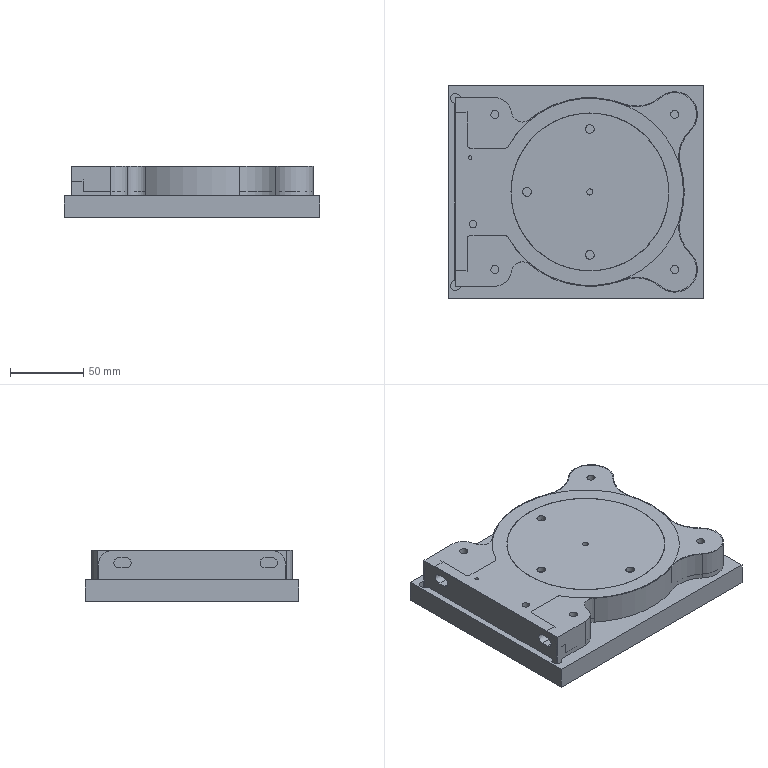NC program | NX | posted with a generic post | part box 175 x 146 x 35 mm
Lines 7000 to 8019 of 35144:
(深度开粗_COPY_COPY_1 , TOOL : D3)
N13836 T06 M6
N13838 G54
N13840 G17 G0 G90 X-69.928 Y23. S9000 M3
N13842 G43 Z20. H6
N13844 Z0.102
N13846 G94 G1 Z-0.398 F2500.
N13848 G3 X-71.428 Y24.5 R1.5
N13850 G1 X-72.5
N13852 G3 X-73. Y24. R0.5
N13854 G1 Y22.928
N13856 G3 X-71.5 Y21.428 R1.5
N13858 G1 Z0.102
N13860 G0 X-69.928 Y23. Z-0.296
N13862 G1 Z-0.796
N13864 G3 X-71.428 Y24.5 R1.5
N13866 G1 X-72.5
N13868 G3 X-73. Y24. R0.5
N13870 G1 Y22.928
N13872 G3 X-71.5 Y21.428 R1.5
N13874 G1 Z-0.296
N13876 G0 X-69.928 Y23. Z-0.694
N13878 G1 Z-1.194
N13880 G3 X-71.428 Y24.5 R1.5
N13882 G1 X-72.5
N13884 G3 X-73. Y24. R0.5
N13886 G1 Y22.928
N13888 G3 X-71.5 Y21.428 R1.5
N13890 G1 Z-0.694
N13892 G0 X-69.928 Y23. Z-1.092
N13894 G1 Z-1.592
N13896 G3 X-71.428 Y24.5 R1.5
N13898 G1 X-72.5
N13900 G3 X-73. Y24. R0.5
N13902 G1 Y22.928
N13904 G3 X-71.5 Y21.428 R1.5
N13906 G1 Z-1.092
N13908 G0 X-69.928 Y23. Z-1.49
N13910 G1 Z-1.99
N13912 G3 X-71.428 Y24.5 R1.5
N13914 G1 X-72.5
N13916 G3 X-73. Y24. R0.5
N13918 G1 Y22.928
N13920 G3 X-71.5 Y21.428 R1.5
N13922 G1 Z-1.49
N13924 G0 X-69.928 Y23. Z-1.888
N13926 G1 Z-2.388
N13928 G3 X-71.428 Y24.5 R1.5
N13930 G1 X-72.5
N13932 G3 X-73. Y24. R0.5
N13934 G1 Y22.928
N13936 G3 X-71.5 Y21.428 R1.5
N13938 G1 Z-1.888
N13940 G0 X-69.928 Y23. Z-2.286
N13942 G1 Z-2.786
N13944 G3 X-71.428 Y24.5 R1.5
N13946 G1 X-72.5
N13948 G3 X-73. Y24. R0.5
N13950 G1 Y22.928
N13952 G3 X-71.5 Y21.428 R1.5
N13954 G1 Z-2.286
N13956 G0 X-69.928 Y23. Z-2.684
N13958 G1 Z-3.184
N13960 G3 X-71.428 Y24.5 R1.5
N13962 G1 X-72.5
N13964 G3 X-73. Y24. R0.5
N13966 G1 Y22.928
N13968 G3 X-71.5 Y21.428 R1.5
N13970 G1 Z-2.684
N13972 G0 X-69.928 Y23. Z-3.082
N13974 G1 Z-3.582
N13976 G3 X-71.428 Y24.5 R1.5
N13978 G1 X-72.5
N13980 G3 X-73. Y24. R0.5
N13982 G1 Y22.928
N13984 G3 X-71.5 Y21.428 R1.5
N13986 G1 Z-3.082
N13988 G0 X-69.928 Y23. Z-3.48
N13990 G1 Z-3.98
N13992 G3 X-71.428 Y24.5 R1.5
N13994 G1 X-72.5
N13996 G3 X-73. Y24. R0.5
N13998 G1 Y22.928
N14000 G3 X-71.5 Y21.428 R1.5
N14002 G1 Z-3.48
N14004 G0 X-69.928 Y23. Z-3.878
N14006 G1 Z-4.378
N14008 G3 X-71.428 Y24.5 R1.5
N14010 G1 X-72.5
N14012 G3 X-73. Y24. R0.5
N14014 G1 Y22.928
N14016 G3 X-71.5 Y21.428 R1.5
N14018 G1 Z-3.878
N14020 G0 X-69.928 Y23. Z-4.276
N14022 G1 Z-4.776
N14024 G3 X-71.428 Y24.5 R1.5
N14026 G1 X-72.5
N14028 G3 X-73. Y24. R0.5
N14030 G1 Y22.928
N14032 G3 X-71.5 Y21.428 R1.5
N14034 G1 Z-4.276
N14036 G0 X-69.928 Y23. Z-4.675
N14038 G1 Z-5.175
N14040 G3 X-71.428 Y24.5 R1.5
N14042 G1 X-72.5
N14044 G3 X-73. Y24. R0.5
N14046 G1 Y22.928
N14048 G3 X-71.5 Y21.428 R1.5
N14050 G1 Z-4.675
N14052 G0 X-69.928 Y23. Z-5.073
N14054 G1 Z-5.573
N14056 G3 X-71.428 Y24.5 R1.5
N14058 G1 X-72.5
N14060 G3 X-73. Y24. R0.5
N14062 G1 Y22.928
N14064 G3 X-71.5 Y21.428 R1.5
N14066 G1 Z-5.073
N14068 G0 X-69.928 Y23. Z-5.471
N14070 G1 Z-5.971
N14072 G3 X-71.428 Y24.5 R1.5
N14074 G1 X-72.5
N14076 G3 X-73. Y24. R0.5
N14078 G1 Y22.928
N14080 G3 X-71.5 Y21.428 R1.5
N14082 G1 Z-5.471
N14084 G0 X-69.928 Y23. Z-5.869
N14086 G1 Z-6.369
N14088 G3 X-71.428 Y24.5 R1.5
N14090 G1 X-72.5
N14092 G3 X-73. Y24. R0.5
N14094 G1 Y22.928
N14096 G3 X-71.5 Y21.428 R1.5
N14098 G1 Z-5.869
N14100 G0 X-69.928 Y23. Z-6.267
N14102 G1 Z-6.767
N14104 G3 X-71.428 Y24.5 R1.5
N14106 G1 X-72.5
N14108 G3 X-73. Y24. R0.5
N14110 G1 Y22.928
N14112 G3 X-71.5 Y21.428 R1.5
N14114 G1 Z-6.267
N14116 G0 X-69.928 Y23. Z-6.665
N14118 G1 Z-7.165
N14120 G3 X-71.428 Y24.5 R1.5
N14122 G1 X-72.5
N14124 G3 X-73. Y24. R0.5
N14126 G1 Y22.928
N14128 G3 X-71.5 Y21.428 R1.5
N14130 G1 Z-6.665
N14132 G0 X-69.928 Y23. Z-7.063
N14134 G1 Z-7.563
N14136 G3 X-71.428 Y24.5 R1.5
N14138 G1 X-72.5
N14140 G3 X-73. Y24. R0.5
N14142 G1 Y22.928
N14144 G3 X-71.5 Y21.428 R1.5
N14146 G1 Z-7.063
N14148 G0 X-69.928 Y23. Z-7.461
N14150 G1 Z-7.961
N14152 G3 X-71.428 Y24.5 R1.5
N14154 G1 X-72.5
N14156 G3 X-73. Y24. R0.5
N14158 G1 Y22.928
N14160 G3 X-71.5 Y21.428 R1.5
N14162 G1 Z-7.461
N14164 G0 X-69.928 Y23. Z-7.859
N14166 G1 Z-8.359
N14168 G3 X-71.428 Y24.5 R1.5
N14170 G1 X-72.5
N14172 G3 X-73. Y24. R0.5
N14174 G1 Y22.928
N14176 G3 X-71.5 Y21.428 R1.5
N14178 G1 Z-7.859
N14180 G0 X-69.928 Y23. Z-8.257
N14182 G1 Z-8.757
N14184 G3 X-71.428 Y24.5 R1.5
N14186 G1 X-72.5
N14188 G3 X-73. Y24. R0.5
N14190 G1 Y22.928
N14192 G3 X-71.5 Y21.428 R1.5
N14194 G1 Z-8.257
N14196 G0 X-69.928 Y23. Z-8.655
N14198 G1 Z-9.155
N14200 G3 X-71.428 Y24.5 R1.5
N14202 G1 X-72.5
N14204 G3 X-73. Y24. R0.5
N14206 G1 Y22.928
N14208 G3 X-71.5 Y21.428 R1.5
N14210 G1 Z-8.655
N14212 G0 X-69.928 Y23. Z-9.053
N14214 G1 Z-9.553
N14216 G3 X-71.428 Y24.5 R1.5
N14218 G1 X-72.5
N14220 G3 X-73. Y24. R0.5
N14222 G1 Y22.928
N14224 G3 X-71.5 Y21.428 R1.5
N14226 G1 Z-9.053
N14228 G0 X-69.928 Y23. Z-9.451
N14230 G1 Z-9.951
N14232 G3 X-71.428 Y24.5 R1.5
N14234 G1 X-72.5
N14236 G3 X-73. Y24. R0.5
N14238 G1 Y22.928
N14240 G3 X-71.5 Y21.428 R1.5
N14242 G1 Z-9.451
N14244 G0 X-69.928 Y23. Z-9.849
N14246 G1 Z-10.349
N14248 G3 X-71.428 Y24.5 R1.5
N14250 G1 X-72.5
N14252 G3 X-73. Y24. R0.5
N14254 G1 Y22.928
N14256 G3 X-71.5 Y21.428 R1.5
N14258 G1 Z-9.849
N14260 G0 X-69.928 Y23. Z-10.247
N14262 G1 Z-10.747
N14264 G3 X-71.428 Y24.5 R1.5
N14266 G1 X-72.5
N14268 G3 X-73. Y24. R0.5
N14270 G1 Y22.928
N14272 G3 X-71.5 Y21.428 R1.5
N14274 G1 Z-10.247
N14276 G0 X-69.928 Y23. Z-10.645
N14278 G1 Z-11.145
N14280 G3 X-71.428 Y24.5 R1.5
N14282 G1 X-72.5
N14284 G3 X-73. Y24. R0.5
N14286 G1 Y22.928
N14288 G3 X-71.5 Y21.428 R1.5
N14290 G1 Z-10.645
N14292 G0 X-69.928 Y23. Z-11.043
N14294 G1 Z-11.543
N14296 G3 X-71.428 Y24.5 R1.5
N14298 G1 X-72.5
N14300 G3 X-73. Y24. R0.5
N14302 G1 Y22.928
N14304 G3 X-71.5 Y21.428 R1.5
N14306 G1 Z-11.043
N14308 G0 X-69.928 Y23. Z-11.441
N14310 G1 Z-11.941
N14312 G3 X-71.428 Y24.5 R1.5
N14314 G1 X-72.5
N14316 G3 X-73. Y24. R0.5
N14318 G1 Y22.928
N14320 G3 X-71.5 Y21.428 R1.5
N14322 G1 Z-11.441
N14324 G0 X-69.928 Y23. Z-11.839
N14326 G1 Z-12.339
N14328 G3 X-71.428 Y24.5 R1.5
N14330 G1 X-72.5
N14332 G3 X-73. Y24. R0.5
N14334 G1 Y22.928
N14336 G3 X-71.5 Y21.428 R1.5
N14338 G1 Z-11.839
N14340 G0 X-69.928 Y23. Z-12.237
N14342 G1 Z-12.737
N14344 G3 X-71.428 Y24.5 R1.5
N14346 G1 X-72.5
N14348 G3 X-73. Y24. R0.5
N14350 G1 Y22.928
N14352 G3 X-71.5 Y21.428 R1.5
N14354 G1 Z-12.237
N14356 G0 X-69.928 Y23. Z-12.635
N14358 G1 Z-13.135
N14360 G3 X-71.428 Y24.5 R1.5
N14362 G1 X-72.5
N14364 G3 X-73. Y24. R0.5
N14366 G1 Y22.928
N14368 G3 X-71.5 Y21.428 R1.5
N14370 G1 Z-12.635
N14372 G0 X-69.928 Y23. Z-13.033
N14374 G1 Z-13.533
N14376 G3 X-71.428 Y24.5 R1.5
N14378 G1 X-72.5
N14380 G3 X-73. Y24. R0.5
N14382 G1 Y22.928
N14384 G3 X-71.5 Y21.428 R1.5
N14386 G1 Z-13.033
N14388 G0 X-69.928 Y23. Z-13.431
N14390 G1 Z-13.931
N14392 G3 X-71.428 Y24.5 R1.5
N14394 G1 X-72.5
N14396 G3 X-73. Y24. R0.5
N14398 G1 Y22.928
N14400 G3 X-71.5 Y21.428 R1.5
N14402 G1 Z-13.431
N14404 G0 X-69.928 Y23. Z-13.829
N14406 G1 Z-14.329
N14408 G3 X-71.428 Y24.5 R1.5
N14410 G1 X-72.5
N14412 G3 X-73. Y24. R0.5
N14414 G1 Y22.928
N14416 G3 X-71.5 Y21.428 R1.5
N14418 G1 Z-13.829
N14420 G0 X-69.928 Y23. Z-14.227
N14422 G1 Z-14.727
N14424 G3 X-71.428 Y24.5 R1.5
N14426 G1 X-72.5
N14428 G3 X-73. Y24. R0.5
N14430 G1 Y22.928
N14432 G3 X-71.5 Y21.428 R1.5
N14434 G1 Z-14.227
N14436 G0 X-69.928 Y23. Z-14.625
N14438 G1 Z-15.125
N14440 G3 X-71.428 Y24.5 R1.5
N14442 G1 X-72.5
N14444 G3 X-73. Y24. R0.5
N14446 G1 Y22.928
N14448 G3 X-71.5 Y21.428 R1.5
N14450 G1 Z-14.625
N14452 G0 X-69.928 Y23. Z-15.024
N14454 G1 Z-15.524
N14456 G3 X-71.428 Y24.5 R1.5
N14458 G1 X-72.5
N14460 G3 X-73. Y24. R0.5
N14462 G1 Y22.928
N14464 G3 X-71.5 Y21.428 R1.5
N14466 G1 Z-15.024
N14468 G0 X-69.928 Y23. Z-15.422
N14470 G1 Z-15.922
N14472 G3 X-71.428 Y24.5 R1.5
N14474 G1 X-72.5
N14476 G3 X-73. Y24. R0.5
N14478 G1 Y22.928
N14480 G3 X-71.5 Y21.428 R1.5
N14482 G1 Z-15.422
N14484 G0 X-69.928 Y23. Z-15.82
N14486 G1 Z-16.32
N14488 G3 X-71.428 Y24.5 R1.5
N14490 G1 X-72.5
N14492 G3 X-73. Y24. R0.5
N14494 G1 Y22.928
N14496 G3 X-71.5 Y21.428 R1.5
N14498 G1 Z-15.82
N14500 G0 X-69.928 Y23. Z-16.218
N14502 G1 Z-16.718
N14504 G3 X-71.428 Y24.5 R1.5
N14506 G1 X-72.5
N14508 G3 X-73. Y24. R0.5
N14510 G1 Y22.928
N14512 G3 X-71.5 Y21.428 R1.5
N14514 G1 Z-16.218
N14516 G0 X-69.928 Y23. Z-16.616
N14518 G1 Z-17.116
N14520 G3 X-71.428 Y24.5 R1.5
N14522 G1 X-72.5
N14524 G3 X-73. Y24. R0.5
N14526 G1 Y22.928
N14528 G3 X-71.5 Y21.428 R1.5
N14530 G1 Z-16.616
N14532 G0 X-69.928 Y23. Z-17.014
N14534 G1 Z-17.514
N14536 G3 X-71.428 Y24.5 R1.5
N14538 G1 X-72.5
N14540 G3 X-73. Y24. R0.5
N14542 G1 Y22.928
N14544 G3 X-71.5 Y21.428 R1.5
N14546 G1 Z-17.014
N14548 G0 X-69.928 Y23. Z-17.412
N14550 G1 Z-17.912
N14552 G3 X-71.428 Y24.5 R1.5
N14554 G1 X-72.5
N14556 G3 X-73. Y24. R0.5
N14558 G1 Y22.928
N14560 G3 X-71.5 Y21.428 R1.5
N14562 G1 Z-17.412
N14564 G0 X-69.928 Y23. Z-17.81
N14566 G1 Z-18.31
N14568 G3 X-71.428 Y24.5 R1.5
N14570 G1 X-72.5
N14572 G3 X-73. Y24. R0.5
N14574 G1 Y22.928
N14576 G3 X-71.5 Y21.428 R1.5
N14578 G1 Z-17.81
N14580 G0 X-69.928 Y23. Z-18.208
N14582 G1 Z-18.708
N14584 G3 X-71.428 Y24.5 R1.5
N14586 G1 X-72.5
N14588 G3 X-73. Y24. R0.5
N14590 G1 Y22.928
N14592 G3 X-71.5 Y21.428 R1.5
N14594 G1 Z-18.208
N14596 G0 X-69.928 Y23. Z-18.606
N14598 G1 Z-19.106
N14600 G3 X-71.428 Y24.5 R1.5
N14602 G1 X-72.5
N14604 G3 X-73. Y24. R0.5
N14606 G1 Y22.928
N14608 G3 X-71.5 Y21.428 R1.5
N14610 G1 Z-18.606
N14612 G0 X-69.928 Y23. Z-19.004
N14614 G1 Z-19.504
N14616 G3 X-71.428 Y24.5 R1.5
N14618 G1 X-72.5
N14620 G3 X-73. Y24. R0.5
N14622 G1 Y22.928
N14624 G3 X-71.5 Y21.428 R1.5
N14626 G1 Z-19.004
N14628 G0 X-69.928 Y23. Z-19.402
N14630 G1 Z-19.902
N14632 G3 X-71.428 Y24.5 R1.5
N14634 G1 X-72.5
N14636 G3 X-73. Y24. R0.5
N14638 G1 Y22.928
N14640 G3 X-71.5 Y21.428 R1.5
N14642 G1 Z-19.402
N14644 G0 X-69.928 Y23. Z-19.8
N14646 G1 Z-20.3
N14648 G3 X-71.428 Y24.5 R1.5
N14650 G1 X-72.5
N14652 G3 X-73. Y24. R0.5
N14654 G1 Y22.928
N14656 G3 X-71.5 Y21.428 R1.5
N14658 G1 Z-19.8
N14660 G0 Z20.
N14662 Y-21.428
N14664 Z0.102
N14666 G1 Z-0.398
N14668 G3 X-73. Y-22.928 R1.5
N14670 G1 Y-24.5
N14672 X-71.428
N14674 G3 X-69.928 Y-23. R1.5
N14676 G1 Z0.102
N14678 G0 X-71.5 Y-21.428 Z-0.296
N14680 G1 Z-0.796
N14682 G3 X-73. Y-22.928 R1.5
N14684 G1 Y-24.5
N14686 X-71.428
N14688 G3 X-69.928 Y-23. R1.5
N14690 G1 Z-0.296
N14692 G0 X-71.5 Y-21.428 Z-0.694
N14694 G1 Z-1.194
N14696 G3 X-73. Y-22.928 R1.5
N14698 G1 Y-24.5
N14700 X-71.428
N14702 G3 X-69.928 Y-23. R1.5
N14704 G1 Z-0.694
N14706 G0 X-71.5 Y-21.428 Z-1.092
N14708 G1 Z-1.592
N14710 G3 X-73. Y-22.928 R1.5
N14712 G1 Y-24.5
N14714 X-71.428
N14716 G3 X-69.928 Y-23. R1.5
N14718 G1 Z-1.092
N14720 G0 X-71.5 Y-21.428 Z-1.49
N14722 G1 Z-1.99
N14724 G3 X-73. Y-22.928 R1.5
N14726 G1 Y-24.5
N14728 X-71.428
N14730 G3 X-69.928 Y-23. R1.5
N14732 G1 Z-1.49
N14734 G0 X-71.5 Y-21.428 Z-1.888
N14736 G1 Z-2.388
N14738 G3 X-73. Y-22.928 R1.5
N14740 G1 Y-24.5
N14742 X-71.428
N14744 G3 X-69.928 Y-23. R1.5
N14746 G1 Z-1.888
N14748 G0 X-71.5 Y-21.428 Z-2.286
N14750 G1 Z-2.786
N14752 G3 X-73. Y-22.928 R1.5
N14754 G1 Y-24.5
N14756 X-71.428
N14758 G3 X-69.928 Y-23. R1.5
N14760 G1 Z-2.286
N14762 G0 X-71.5 Y-21.428 Z-2.684
N14764 G1 Z-3.184
N14766 G3 X-73. Y-22.928 R1.5
N14768 G1 Y-24.5
N14770 X-71.428
N14772 G3 X-69.928 Y-23. R1.5
N14774 G1 Z-2.684
N14776 G0 X-71.5 Y-21.428 Z-3.082
N14778 G1 Z-3.582
N14780 G3 X-73. Y-22.928 R1.5
N14782 G1 Y-24.5
N14784 X-71.428
N14786 G3 X-69.928 Y-23. R1.5
N14788 G1 Z-3.082
N14790 G0 X-71.5 Y-21.428 Z-3.48
N14792 G1 Z-3.98
N14794 G3 X-73. Y-22.928 R1.5
N14796 G1 Y-24.5
N14798 X-71.428
N14800 G3 X-69.928 Y-23. R1.5
N14802 G1 Z-3.48
N14804 G0 X-71.5 Y-21.428 Z-3.878
N14806 G1 Z-4.378
N14808 G3 X-73. Y-22.928 R1.5
N14810 G1 Y-24.5
N14812 X-71.428
N14814 G3 X-69.928 Y-23. R1.5
N14816 G1 Z-3.878
N14818 G0 X-71.5 Y-21.428 Z-4.276
N14820 G1 Z-4.776
N14822 G3 X-73. Y-22.928 R1.5
N14824 G1 Y-24.5
N14826 X-71.428
N14828 G3 X-69.928 Y-23. R1.5
N14830 G1 Z-4.276
N14832 G0 X-71.5 Y-21.428 Z-4.675
N14834 G1 Z-5.175
N14836 G3 X-73. Y-22.928 R1.5
N14838 G1 Y-24.5
N14840 X-71.428
N14842 G3 X-69.928 Y-23. R1.5
N14844 G1 Z-4.675
N14846 G0 X-71.5 Y-21.428 Z-5.073
N14848 G1 Z-5.573
N14850 G3 X-73. Y-22.928 R1.5
N14852 G1 Y-24.5
N14854 X-71.428
N14856 G3 X-69.928 Y-23. R1.5
N14858 G1 Z-5.073
N14860 G0 X-71.5 Y-21.428 Z-5.471
N14862 G1 Z-5.971
N14864 G3 X-73. Y-22.928 R1.5
N14866 G1 Y-24.5
N14868 X-71.428
N14870 G3 X-69.928 Y-23. R1.5
N14872 G1 Z-5.471
N14874 G0 X-71.5 Y-21.428 Z-5.869
N14876 G1 Z-6.369
N14878 G3 X-73. Y-22.928 R1.5
N14880 G1 Y-24.5
N14882 X-71.428
N14884 G3 X-69.928 Y-23. R1.5
N14886 G1 Z-5.869
N14888 G0 X-71.5 Y-21.428 Z-6.267
N14890 G1 Z-6.767
N14892 G3 X-73. Y-22.928 R1.5
N14894 G1 Y-24.5
N14896 X-71.428
N14898 G3 X-69.928 Y-23. R1.5
N14900 G1 Z-6.267
N14902 G0 X-71.5 Y-21.428 Z-6.665
N14904 G1 Z-7.165
N14906 G3 X-73. Y-22.928 R1.5
N14908 G1 Y-24.5
N14910 X-71.428
N14912 G3 X-69.928 Y-23. R1.5
N14914 G1 Z-6.665
N14916 G0 X-71.5 Y-21.428 Z-7.063
N14918 G1 Z-7.563
N14920 G3 X-73. Y-22.928 R1.5
N14922 G1 Y-24.5
N14924 X-71.428
N14926 G3 X-69.928 Y-23. R1.5
N14928 G1 Z-7.063
N14930 G0 X-71.5 Y-21.428 Z-7.461
N14932 G1 Z-7.961
N14934 G3 X-73. Y-22.928 R1.5
N14936 G1 Y-24.5
N14938 X-71.428
N14940 G3 X-69.928 Y-23. R1.5
N14942 G1 Z-7.461
N14944 G0 X-71.5 Y-21.428 Z-7.859
N14946 G1 Z-8.359
N14948 G3 X-73. Y-22.928 R1.5
N14950 G1 Y-24.5
N14952 X-71.428
N14954 G3 X-69.928 Y-23. R1.5
N14956 G1 Z-7.859
N14958 G0 X-71.5 Y-21.428 Z-8.257
N14960 G1 Z-8.757
N14962 G3 X-73. Y-22.928 R1.5
N14964 G1 Y-24.5
N14966 X-71.428
N14968 G3 X-69.928 Y-23. R1.5
N14970 G1 Z-8.257
N14972 G0 X-71.5 Y-21.428 Z-8.655
N14974 G1 Z-9.155
N14976 G3 X-73. Y-22.928 R1.5
N14978 G1 Y-24.5
N14980 X-71.428
N14982 G3 X-69.928 Y-23. R1.5
N14984 G1 Z-8.655
N14986 G0 X-71.5 Y-21.428 Z-9.053
N14988 G1 Z-9.553
N14990 G3 X-73. Y-22.928 R1.5
N14992 G1 Y-24.5
N14994 X-71.428
N14996 G3 X-69.928 Y-23. R1.5
N14998 G1 Z-9.053
N15000 G0 X-71.5 Y-21.428 Z-9.451
N15002 G1 Z-9.951
N15004 G3 X-73. Y-22.928 R1.5
N15006 G1 Y-24.5
N15008 X-71.428
N15010 G3 X-69.928 Y-23. R1.5
N15012 G1 Z-9.451
N15014 G0 X-71.5 Y-21.428 Z-9.849
N15016 G1 Z-10.349
N15018 G3 X-73. Y-22.928 R1.5
N15020 G1 Y-24.5
N15022 X-71.428
N15024 G3 X-69.928 Y-23. R1.5
N15026 G1 Z-9.849
N15028 G0 X-71.5 Y-21.428 Z-10.247
N15030 G1 Z-10.747
N15032 G3 X-73. Y-22.928 R1.5
N15034 G1 Y-24.5
N15036 X-71.428
N15038 G3 X-69.928 Y-23. R1.5
N15040 G1 Z-10.247
N15042 G0 X-71.5 Y-21.428 Z-10.645
N15044 G1 Z-11.145
N15046 G3 X-73. Y-22.928 R1.5
N15048 G1 Y-24.5
N15050 X-71.428
N15052 G3 X-69.928 Y-23. R1.5
N15054 G1 Z-10.645
N15056 G0 X-71.5 Y-21.428 Z-11.043
N15058 G1 Z-11.543
N15060 G3 X-73. Y-22.928 R1.5
N15062 G1 Y-24.5
N15064 X-71.428
N15066 G3 X-69.928 Y-23. R1.5
N15068 G1 Z-11.043
N15070 G0 X-71.5 Y-21.428 Z-11.441
N15072 G1 Z-11.941
N15074 G3 X-73. Y-22.928 R1.5
N15076 G1 Y-24.5
N15078 X-71.428
N15080 G3 X-69.928 Y-23. R1.5
N15082 G1 Z-11.441
N15084 G0 X-71.5 Y-21.428 Z-11.839
N15086 G1 Z-12.339
N15088 G3 X-73. Y-22.928 R1.5
N15090 G1 Y-24.5
N15092 X-71.428
N15094 G3 X-69.928 Y-23. R1.5
N15096 G1 Z-11.839
N15098 G0 X-71.5 Y-21.428 Z-12.237
N15100 G1 Z-12.737
N15102 G3 X-73. Y-22.928 R1.5
N15104 G1 Y-24.5
N15106 X-71.428
N15108 G3 X-69.928 Y-23. R1.5
N15110 G1 Z-12.237
N15112 G0 X-71.5 Y-21.428 Z-12.635
N15114 G1 Z-13.135
N15116 G3 X-73. Y-22.928 R1.5
N15118 G1 Y-24.5
N15120 X-71.428
N15122 G3 X-69.928 Y-23. R1.5
N15124 G1 Z-12.635
N15126 G0 X-71.5 Y-21.428 Z-13.033
N15128 G1 Z-13.533
N15130 G3 X-73. Y-22.928 R1.5
N15132 G1 Y-24.5
N15134 X-71.428
N15136 G3 X-69.928 Y-23. R1.5
N15138 G1 Z-13.033
N15140 G0 X-71.5 Y-21.428 Z-13.431
N15142 G1 Z-13.931
N15144 G3 X-73. Y-22.928 R1.5
N15146 G1 Y-24.5
N15148 X-71.428
N15150 G3 X-69.928 Y-23. R1.5
N15152 G1 Z-13.431
N15154 G0 X-71.5 Y-21.428 Z-13.829
N15156 G1 Z-14.329
N15158 G3 X-73. Y-22.928 R1.5
N15160 G1 Y-24.5
N15162 X-71.428
N15164 G3 X-69.928 Y-23. R1.5
N15166 G1 Z-13.829
N15168 G0 X-71.5 Y-21.428 Z-14.227
N15170 G1 Z-14.727
N15172 G3 X-73. Y-22.928 R1.5
N15174 G1 Y-24.5
N15176 X-71.428
N15178 G3 X-69.928 Y-23. R1.5
N15180 G1 Z-14.227
N15182 G0 X-71.5 Y-21.428 Z-14.625
N15184 G1 Z-15.125
N15186 G3 X-73. Y-22.928 R1.5
N15188 G1 Y-24.5
N15190 X-71.428
N15192 G3 X-69.928 Y-23. R1.5
N15194 G1 Z-14.625
N15196 G0 X-71.5 Y-21.428 Z-15.024
N15198 G1 Z-15.524
N15200 G3 X-73. Y-22.928 R1.5
N15202 G1 Y-24.5
N15204 X-71.428
N15206 G3 X-69.928 Y-23. R1.5
N15208 G1 Z-15.024
N15210 G0 X-71.5 Y-21.428 Z-15.422
N15212 G1 Z-15.922
N15214 G3 X-73. Y-22.928 R1.5
N15216 G1 Y-24.5
N15218 X-71.428
N15220 G3 X-69.928 Y-23. R1.5
N15222 G1 Z-15.422
N15224 G0 X-71.5 Y-21.428 Z-15.82
N15226 G1 Z-16.32
N15228 G3 X-73. Y-22.928 R1.5
N15230 G1 Y-24.5
N15232 X-71.428
N15234 G3 X-69.928 Y-23. R1.5
N15236 G1 Z-15.82
N15238 G0 X-71.5 Y-21.428 Z-16.218
N15240 G1 Z-16.718
N15242 G3 X-73. Y-22.928 R1.5
N15244 G1 Y-24.5
N15246 X-71.428
N15248 G3 X-69.928 Y-23. R1.5
N15250 G1 Z-16.218
N15252 G0 X-71.5 Y-21.428 Z-16.616
N15254 G1 Z-17.116
N15256 G3 X-73. Y-22.928 R1.5
N15258 G1 Y-24.5
N15260 X-71.428
N15262 G3 X-69.928 Y-23. R1.5
N15264 G1 Z-16.616
N15266 G0 X-71.5 Y-21.428 Z-17.014
N15268 G1 Z-17.514
N15270 G3 X-73. Y-22.928 R1.5
N15272 G1 Y-24.5
N15274 X-71.428
N15276 G3 X-69.928 Y-23. R1.5
N15278 G1 Z-17.014
N15280 G0 X-71.5 Y-21.428 Z-17.412
N15282 G1 Z-17.912
N15284 G3 X-73. Y-22.928 R1.5
N15286 G1 Y-24.5
N15288 X-71.428
N15290 G3 X-69.928 Y-23. R1.5
N15292 G1 Z-17.412
N15294 G0 X-71.5 Y-21.428 Z-17.81
N15296 G1 Z-18.31
N15298 G3 X-73. Y-22.928 R1.5
N15300 G1 Y-24.5
N15302 X-71.428
N15304 G3 X-69.928 Y-23. R1.5
N15306 G1 Z-17.81
N15308 G0 X-71.5 Y-21.428 Z-18.208
N15310 G1 Z-18.708
N15312 G3 X-73. Y-22.928 R1.5
N15314 G1 Y-24.5
N15316 X-71.428
N15318 G3 X-69.928 Y-23. R1.5
N15320 G1 Z-18.208
N15322 G0 X-71.5 Y-21.428 Z-18.606
N15324 G1 Z-19.106
N15326 G3 X-73. Y-22.928 R1.5
N15328 G1 Y-24.5
N15330 X-71.428
N15332 G3 X-69.928 Y-23. R1.5
N15334 G1 Z-18.606
N15336 G0 X-71.5 Y-21.428 Z-19.004
N15338 G1 Z-19.504
N15340 G3 X-73. Y-22.928 R1.5
N15342 G1 Y-24.5
N15344 X-71.428
N15346 G3 X-69.928 Y-23. R1.5
N15348 G1 Z-19.004
N15350 G0 X-71.5 Y-21.428 Z-19.402
N15352 G1 Z-19.902
N15354 G3 X-73. Y-22.928 R1.5
N15356 G1 Y-24.5
N15358 X-71.428
N15360 G3 X-69.928 Y-23. R1.5
N15362 G1 Z-19.402
N15364 G0 X-71.5 Y-21.428 Z-19.8
N15366 G1 Z-20.3
N15368 G3 X-73. Y-22.928 R1.5
N15370 G1 Y-24.5
N15372 X-71.428
N15374 G3 X-69.928 Y-23. R1.5
N15376 G1 Z-19.8
N15378 G0 X-71.5 Y-21.428 Z-20.15
N15380 G1 Z-20.65
N15382 G3 X-73. Y-22.928 R1.5
N15384 G1 Y-24.5
N15386 X-71.428
N15388 G3 X-69.928 Y-23. R1.5
N15390 G1 Z-20.15
N15392 G0 X-71.5 Y-21.428 Z-20.5
N15394 G1 Z-21.
N15396 G3 X-73. Y-22.928 R1.5
N15398 G1 Y-24.5
N15400 X-71.428
N15402 G3 X-69.928 Y-23. R1.5
N15404 G1 Z-20.5
N15406 G0 X-71.5 Y-21.428 Z-20.857
N15408 G1 Z-21.357
N15410 G3 X-73. Y-22.928 R1.5
N15412 G1 Y-24.5
N15414 X-71.428
N15416 G3 X-69.928 Y-23. R1.5
N15418 G1 Z-20.857
N15420 G0 X-71.5 Y-21.428 Z-21.214
N15422 G1 Z-21.714
N15424 G3 X-73. Y-22.928 R1.5
N15426 G1 Y-24.5
N15428 X-71.428
N15430 G3 X-69.928 Y-23. R1.5
N15432 G1 Z-21.214
N15434 G0 X-71.5 Y-21.428 Z-21.571
N15436 G1 Z-22.071
N15438 G3 X-73. Y-22.928 R1.5
N15440 G1 Y-24.5
N15442 X-71.428
N15444 G3 X-69.928 Y-23. R1.5
N15446 G1 Z-21.571
N15448 G0 X-71.5 Y-21.428 Z-21.929
N15450 G1 Z-22.429
N15452 G3 X-73. Y-22.928 R1.5
N15454 G1 Y-24.5
N15456 X-71.428
N15458 G3 X-69.928 Y-23. R1.5
N15460 G1 Z-21.929
N15462 G0 X-71.5 Y-21.428 Z-22.286
N15464 G1 Z-22.786
N15466 G3 X-73. Y-22.928 R1.5
N15468 G1 Y-24.5
N15470 X-71.428
N15472 G3 X-69.928 Y-23. R1.5
N15474 G1 Z-22.286
N15476 G0 X-71.5 Y-21.428 Z-22.643
N15478 G1 Z-23.143
N15480 G3 X-73. Y-22.928 R1.5
N15482 G1 Y-24.5
N15484 X-71.428
N15486 G3 X-69.928 Y-23. R1.5
N15488 G1 Z-22.643
N15490 G0 X-71.5 Y-21.428 Z-23.
N15492 G1 Z-23.5
N15494 G3 X-73. Y-22.928 R1.5
N15496 G1 Y-24.5
N15498 X-71.428
N15500 G3 X-69.928 Y-23. R1.5
N15502 G1 Z-23.
N15504 G0 Z20.
N15506 Y-22.
N15508 Z-20.857
N15510 G1 Z-21.357
N15512 G3 X-71.428 Y-20.5 R1.5
N15514 G1 X-72.5
N15516 G3 X-73. Y-21. R0.5
N15518 G1 Y-22.072
N15520 G3 X-71.5 Y-23.572 R1.5
N15522 G1 Z-20.857
N15524 G0 X-69.928 Y-22. Z-21.214
N15526 G1 Z-21.714
N15528 G3 X-71.428 Y-20.5 R1.5
N15530 G1 X-72.5
N15532 G3 X-73. Y-21. R0.5
N15534 G1 Y-22.072
N15536 G3 X-71.5 Y-23.572 R1.5
N15538 G1 Z-21.214
N15540 G0 X-69.928 Y-22. Z-21.571
N15542 G1 Z-22.071
N15544 G3 X-71.428 Y-20.5 R1.5
N15546 G1 X-72.5
N15548 G3 X-73. Y-21. R0.5
N15550 G1 Y-22.072
N15552 G3 X-71.5 Y-23.572 R1.5
N15554 G1 Z-21.571
N15556 G0 X-69.928 Y-22. Z-21.929
N15558 G1 Z-22.429
N15560 G3 X-71.428 Y-20.5 R1.5
N15562 G1 X-72.5
N15564 G3 X-73. Y-21. R0.5
N15566 G1 Y-22.072
N15568 G3 X-71.5 Y-23.572 R1.5
N15570 G1 Z-21.929
N15572 G0 X-69.928 Y-22. Z-22.286
N15574 G1 Z-22.786
N15576 G3 X-71.428 Y-20.5 R1.5
N15578 G1 X-72.5
N15580 G3 X-73. Y-21. R0.5
N15582 G1 Y-22.072
N15584 G3 X-71.5 Y-23.572 R1.5
N15586 G1 Z-22.286
N15588 G0 X-69.928 Y-22. Z-22.643
N15590 G1 Z-23.143
N15592 G3 X-71.428 Y-20.5 R1.5
N15594 G1 X-72.5
N15596 G3 X-73. Y-21. R0.5
N15598 G1 Y-22.072
N15600 G3 X-71.5 Y-23.572 R1.5
N15602 G1 Z-22.643
N15604 G0 X-69.928 Y-22. Z-23.
N15606 G1 Z-23.5
N15608 G3 X-71.428 Y-20.5 R1.5
N15610 G1 X-72.5
N15612 G3 X-73. Y-21. R0.5
N15614 G1 Y-22.072
N15616 G3 X-71.5 Y-23.572 R1.5
N15618 G1 Z-23.
N15620 G0 Z20.
N15622 X-70.072 Y-23.
N15624 Z-20.857
N15626 G1 Z-21.357
N15628 G3 X-68.572 Y-24.5 R1.5
N15630 G1 X-67.5
N15632 G3 X-67. Y-24. R0.5
N15634 G1 Y-22.928
N15636 G3 X-68.5 Y-21.428 R1.5
N15638 G1 Z-20.857
N15640 G0 X-70.072 Y-23. Z-21.214
N15642 G1 Z-21.714
N15644 G3 X-68.572 Y-24.5 R1.5
N15646 G1 X-67.5
N15648 G3 X-67. Y-24. R0.5
N15650 G1 Y-22.928
N15652 G3 X-68.5 Y-21.428 R1.5
N15654 G1 Z-21.214
N15656 G0 X-70.072 Y-23. Z-21.571
N15658 G1 Z-22.071
N15660 G3 X-68.572 Y-24.5 R1.5
N15662 G1 X-67.5
N15664 G3 X-67. Y-24. R0.5
N15666 G1 Y-22.928
N15668 G3 X-68.5 Y-21.428 R1.5
N15670 G1 Z-21.571
N15672 G0 X-70.072 Y-23. Z-21.929
N15674 G1 Z-22.429
N15676 G3 X-68.572 Y-24.5 R1.5
N15678 G1 X-67.5
N15680 G3 X-67. Y-24. R0.5
N15682 G1 Y-22.928
N15684 G3 X-68.5 Y-21.428 R1.5
N15686 G1 Z-21.929
N15688 G0 X-70.072 Y-23. Z-22.286
N15690 G1 Z-22.786
N15692 G3 X-68.572 Y-24.5 R1.5
N15694 G1 X-67.5
N15696 G3 X-67. Y-24. R0.5
N15698 G1 Y-22.928
N15700 G3 X-68.5 Y-21.428 R1.5
N15702 G1 Z-22.286
N15704 G0 X-70.072 Y-23. Z-22.643
N15706 G1 Z-23.143
N15708 G3 X-68.572 Y-24.5 R1.5
N15710 G1 X-67.5
N15712 G3 X-67. Y-24. R0.5
N15714 G1 Y-22.928
N15716 G3 X-68.5 Y-21.428 R1.5
N15718 G1 Z-22.643
N15720 G0 X-70.072 Y-23. Z-23.
N15722 G1 Z-23.5
N15724 G3 X-68.572 Y-24.5 R1.5
N15726 G1 X-67.5
N15728 G3 X-67. Y-24. R0.5
N15730 G1 Y-22.928
N15732 G3 X-68.5 Y-21.428 R1.5
N15734 G1 Z-23.
N15736 G0 Z20.
N15738 X-48.928 Y23.
N15740 Z-1.888
N15742 G1 Z-2.388
N15744 G3 X-50.428 Y24.5 R1.5
N15746 G1 X-51.5
N15748 G3 X-52. Y24. R0.5
N15750 G1 Y22.928
N15752 G3 X-50.5 Y21.428 R1.5
N15754 G1 Z-1.888
N15756 G0 X-48.928 Y23. Z-2.286
N15758 G1 Z-2.786
N15760 G3 X-50.428 Y24.5 R1.5
N15762 G1 X-51.5
N15764 G3 X-52. Y24. R0.5
N15766 G1 Y22.928
N15768 G3 X-50.5 Y21.428 R1.5
N15770 G1 Z-2.286
N15772 G0 X-48.928 Y23. Z-2.684
N15774 G1 Z-3.184
N15776 G3 X-50.428 Y24.5 R1.5
N15778 G1 X-51.5
N15780 G3 X-52. Y24. R0.5
N15782 G1 Y22.928
N15784 G3 X-50.5 Y21.428 R1.5
N15786 G1 Z-2.684
N15788 G0 X-48.928 Y23. Z-3.082
N15790 G1 Z-3.582
N15792 G3 X-50.428 Y24.5 R1.5
N15794 G1 X-51.5
N15796 G3 X-52. Y24. R0.5
N15798 G1 Y22.928
N15800 G3 X-50.5 Y21.428 R1.5
N15802 G1 Z-3.082
N15804 G0 X-48.928 Y23. Z-3.48
N15806 G1 Z-3.98
N15808 G3 X-50.428 Y24.5 R1.5
N15810 G1 X-51.5
N15812 G3 X-52. Y24. R0.5
N15814 G1 Y22.928
N15816 G3 X-50.5 Y21.428 R1.5
N15818 G1 Z-3.48
N15820 G0 X-48.928 Y23. Z-3.878
N15822 G1 Z-4.378
N15824 G3 X-50.428 Y24.5 R1.5
N15826 G1 X-51.5
N15828 G3 X-52. Y24. R0.5
N15830 G1 Y22.928
N15832 G3 X-50.5 Y21.428 R1.5
N15834 G1 Z-3.878
N15836 G0 X-48.928 Y23. Z-4.276
N15838 G1 Z-4.776
N15840 G3 X-50.428 Y24.5 R1.5
N15842 G1 X-51.5
N15844 G3 X-52. Y24. R0.5
N15846 G1 Y22.928
N15848 G3 X-50.5 Y21.428 R1.5
N15850 G1 Z-4.276
N15852 G0 X-48.928 Y23. Z-4.675
N15854 G1 Z-5.175
N15856 G3 X-50.428 Y24.5 R1.5
N15858 G1 X-51.5
N15860 G3 X-52. Y24. R0.5
N15862 G1 Y22.928
N15864 G3 X-50.5 Y21.428 R1.5
N15866 G1 Z-4.675
N15868 G0 X-48.928 Y23. Z-5.073